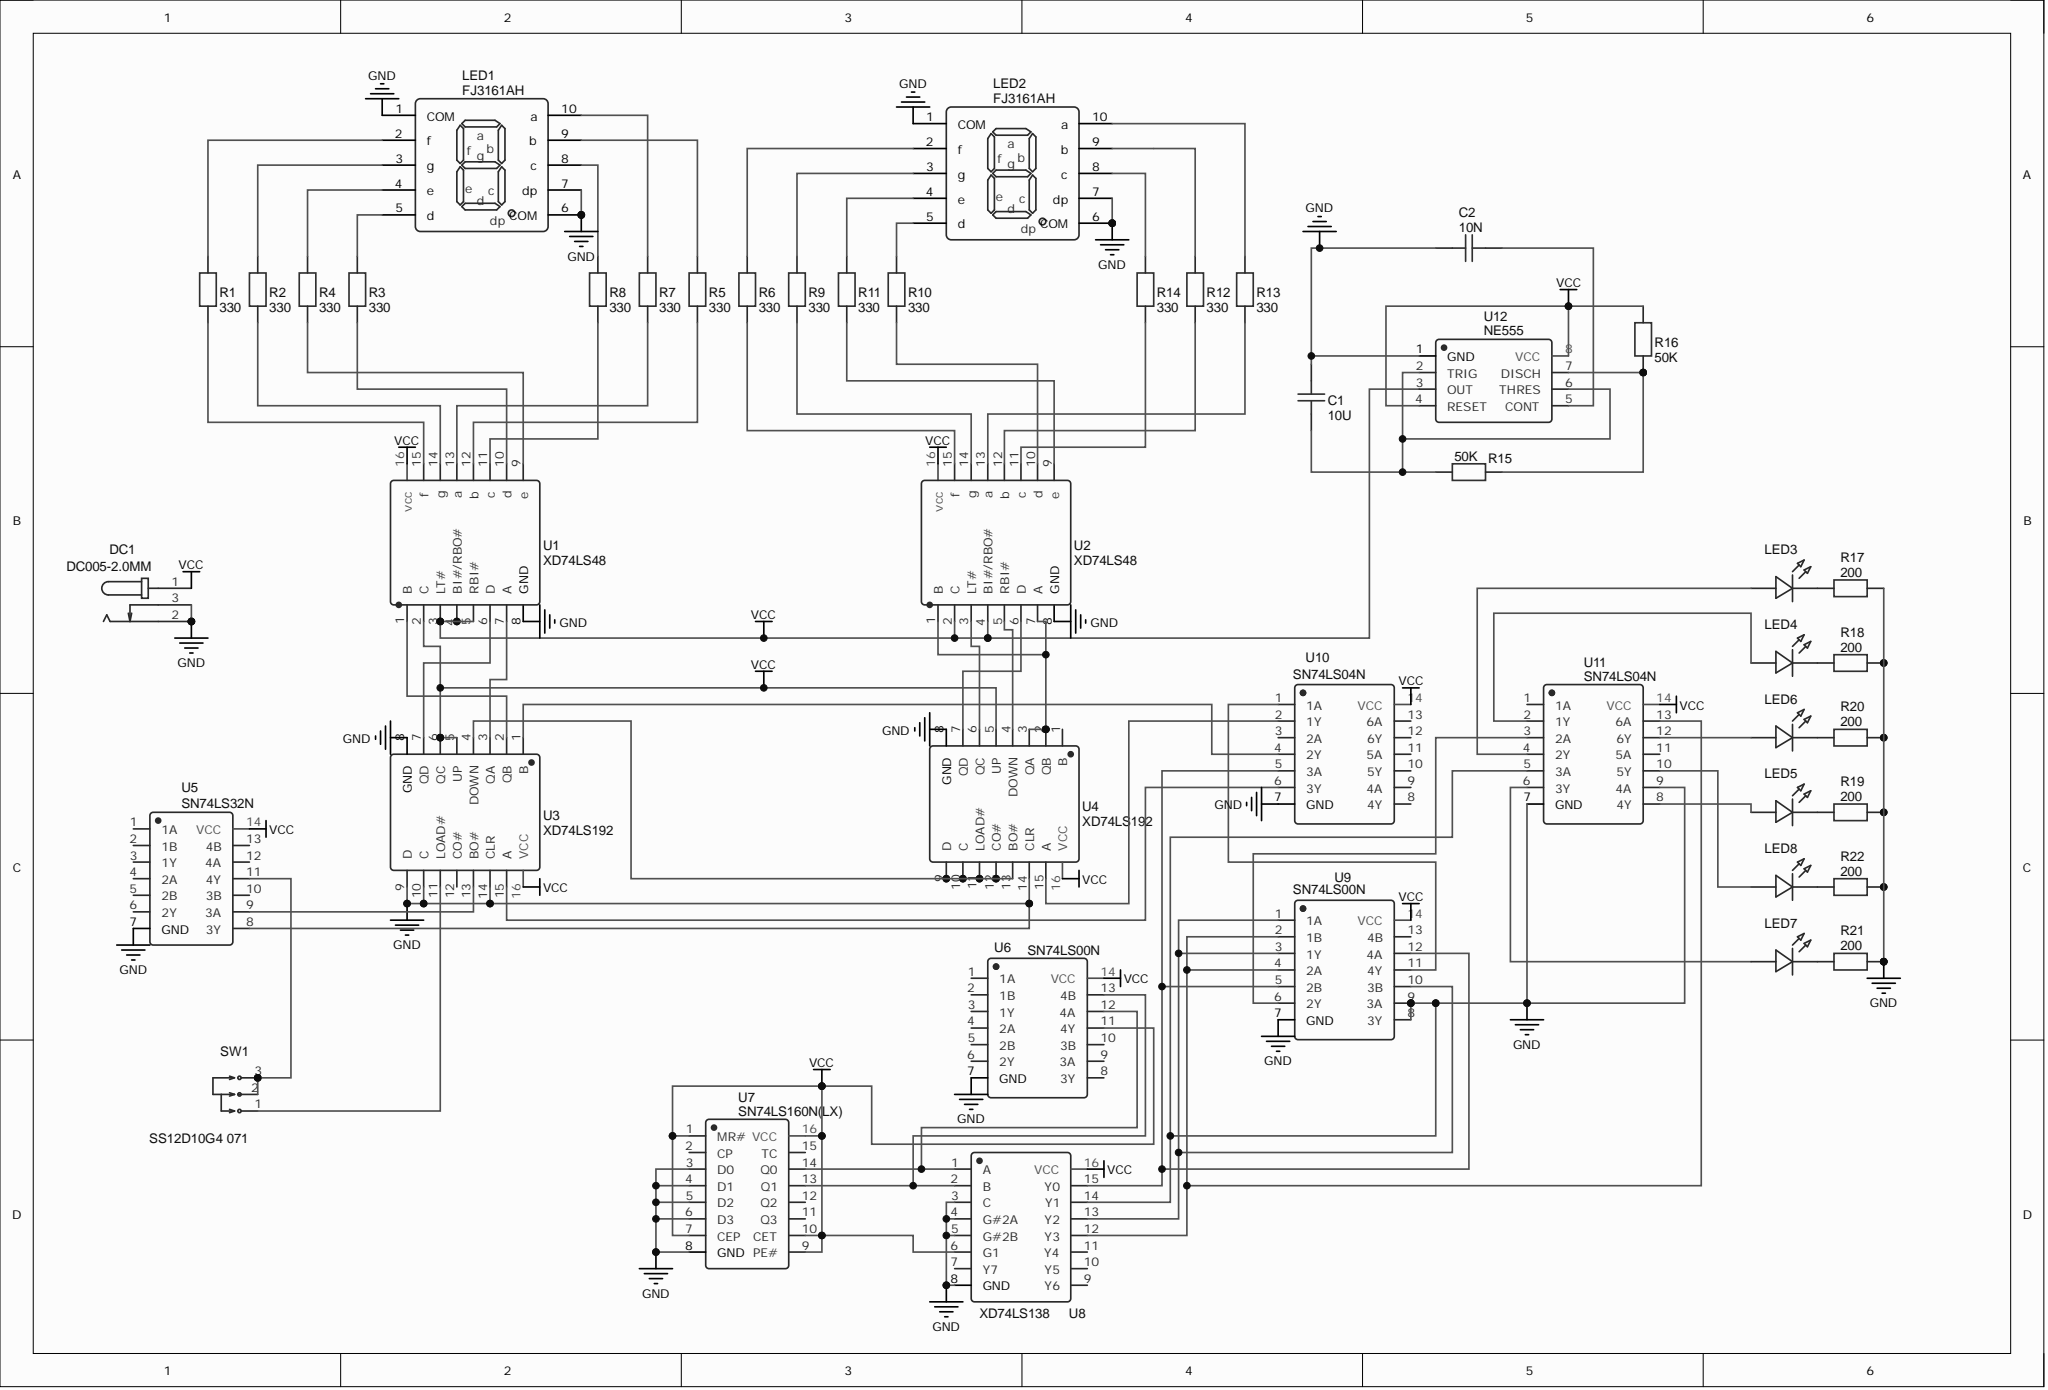Circuit board | Altium Designer | 46 parts | 66 nets
Bill of materials:
Comment,Description,Designator,Footprint,LibRef,Quantity
"10U","","C1","RAD-0.2","10U","1"
"10N","","C2","RAD-0.2","10N","1"
"DC005-2.0MM","","DC1","DC-IN-TH_DC005","DC005-2.0MM","1"
"FJ3161AH","","LED1, LED2","LED-SEG-TH_10P-L14.0-W7.5-P2.54-S5.08-TL","FJ3161AH","2"
"LED-TH-5mm_R","","LED3, LED4, LED5, LED6, LED7, LED8","LED-TH_BD5.0_RED","LED-TH-5mm_R","6"
"330","","R1, R2, R3, R4, R5, R6, R7, R8, R9, R10, R11, R12, R13, R14","R_AXIAL-0.4","330","14"
"50K","","R15, R16","R_AXIAL-0.4","50K","2"
"200","","R17, R18, R19, R20, R21, R22","R_AXIAL-0.4","200","6"
"SS12D10G4 071","","SW1","SW-TH_SHOU-HAN_SS12D10G4","SS12D10G4 071","1"
"XD74LS48","","U1, U2","DIP-16_L19.3-W6.4-P2.54-LS7.6-BL","XD74LS48","2"
"XD74LS192","","U3, U4","DIP-16_L19.3-W6.4-P2.54-LS7.6-BL","XD74LS192","2"
"SN74LS32N","","U5","PDIP-14_L19.6-W6.5-P2.54-LS7.9-BL","SN74LS32N","1"
"SN74LS00N","","U6, U9","PDIP-14_L19.7-W6.6-P2.54-LS8.3-BL","SN74LS00N","2"
"SN74LS160N(LX)","","U7","DIP-16_L22.4-W6.4-P2.54-LS8.64-BL","SN74LS160N(LX)","1"
"XD74LS138","","U8","DIP-16_L19.8-W6.5-P2.54-LS7.6-BL","XD74LS138","1"
"SN74LS04N","","U10, U11","PDIP-14_L19.7-W6.6-P2.54-LS8.3-BL","SN74LS04N","2"
"NE555","","U12","DIP-8_L9.8-W6.6-P2.54-LS7.6-BL","NE555","1"
Netlist (Protel format):
[
C1
RAD-0.2
10U



]
[
C2
RAD-0.2
10N



]
[
DC1
DC-IN-TH_DC005
DC005-2.0MM



]
[
LED1
LED-SEG-TH_10P-L14.0-W7.5-P2.54-S5.08-TL
FJ3161AH



]
[
LED2
LED-SEG-TH_10P-L14.0-W7.5-P2.54-S5.08-TL
FJ3161AH



]
[
LED3
LED-TH_BD5.0_RED
LED-TH-5mm_R



]
[
LED4
LED-TH_BD5.0_RED
LED-TH-5mm_R



]
[
LED5
LED-TH_BD5.0_RED
LED-TH-5mm_R



]
[
LED6
LED-TH_BD5.0_RED
LED-TH-5mm_R



]
[
LED7
LED-TH_BD5.0_RED
LED-TH-5mm_R



]
[
LED8
LED-TH_BD5.0_RED
LED-TH-5mm_R



]
[
R1
R_AXIAL-0.4
330



]
[
R2
R_AXIAL-0.4
330



]
[
R3
R_AXIAL-0.4
330



]
[
R4
R_AXIAL-0.4
330



]
[
R5
R_AXIAL-0.4
330



]
[
R6
R_AXIAL-0.4
330



]
[
R7
R_AXIAL-0.4
330



]
[
R8
R_AXIAL-0.4
330



]
[
R9
R_AXIAL-0.4
330



]
[
R10
R_AXIAL-0.4
330



]
[
R11
R_AXIAL-0.4
330



]
[
R12
R_AXIAL-0.4
330



]
[
R13
R_AXIAL-0.4
330



]
[
R14
R_AXIAL-0.4
330



]
[
R15
R_AXIAL-0.4
50K



]
[
R16
R_AXIAL-0.4
50K



]
[
R17
R_AXIAL-0.4
200



]
[
R18
R_AXIAL-0.4
200



]
[
R19
R_AXIAL-0.4
200



]
[
R20
R_AXIAL-0.4
200



]
[
R21
R_AXIAL-0.4
200



]
[
R22
R_AXIAL-0.4
200



]
[
SW1
SW-TH_SHOU-HAN_SS12D10G4
SS12D10G4 071



]
[
U1
DIP-16_L19.3-W6.4-P2.54-LS7.6-BL
XD74LS48



]
[
U2
DIP-16_L19.3-W6.4-P2.54-LS7.6-BL
XD74LS48



]
[
U3
DIP-16_L19.3-W6.4-P2.54-LS7.6-BL
XD74LS192



]
[
U4
DIP-16_L19.3-W6.4-P2.54-LS7.6-BL
XD74LS192



]
[
U5
PDIP-14_L19.6-W6.5-P2.54-LS7.9-BL
SN74LS32N



]
[
U6
PDIP-14_L19.7-W6.6-P2.54-LS8.3-BL
SN74LS00N



]
[
U7
DIP-16_L22.4-W6.4-P2.54-LS8.64-BL
SN74LS160N(LX)



]
[
U8
DIP-16_L19.8-W6.5-P2.54-LS7.6-BL
XD74LS138



]
[
U9
PDIP-14_L19.7-W6.6-P2.54-LS8.3-BL
SN74LS00N



]
[
U10
PDIP-14_L19.7-W6.6-P2.54-LS8.3-BL
SN74LS04N



]
[
U11
PDIP-14_L19.7-W6.6-P2.54-LS8.3-BL
SN74LS04N



]
[
U12
DIP-8_L9.8-W6.6-P2.54-LS7.6-BL
NE555



]
(
VCC
DC1-1
R16-1
U1-2
U1-3
U1-4
U1-5
U1-16
U2-2
U2-4
U2-16
U3-5
U3-6
U3-16
U4-5
U4-16
U5-14
U6-11
U6-14
U7-1
U7-7
U7-9
U7-10
U7-16
U8-6
U8-16
U9-14
U10-14
U11-14
U12-3
U12-4
U12-8
)
(
NetU9_11
U9-11
U10-1
)
(
NetU9_6
U9-6
U11-3
)
(
NetU8_15
U8-15
U9-5
U9-12
U10-5
)
(
NetU8_13
U8-13
U9-1
U9-3
U9-10
)
(
NetU8_12
U8-12
U9-2
U9-4
U11-13
)
(
NetU6_13
U6-13
U7-13
U8-2
)
(
NetU6_12
U6-12
U7-14
U8-1
)
(
NetU4_15
U4-15
U10-2
)
(
NetU3_15
U3-15
U10-6
)
(
NetU3_13
U3-13
U5-9
)
(
NetU3_4
U3-4
U4-9
U4-10
U4-11
U4-12
U4-13
)
(
NetU3_1
U3-1
U10-4
)
(
NetU2_6
U2-6
U4-7
)
(
NetU2_5
U2-5
U4-4
)
(
NetU2_3
U2-3
U4-6
)
(
NetU2_1
U2-1
U2-7
U4-2
U4-3
)
(
NetU1_7
U1-7
U3-3
)
(
NetU1_6
U1-6
U3-7
)
(
NetU1_1
U1-1
U3-2
)
(
NetSW1_2
SW1-2
SW1-3
U5-11
)
(
NetSW1_1
SW1-1
U3-11
)
(
NetR15_1
R15-1
R16-2
U12-7
)
(
NetR14_1
R14-1
U2-11
)
(
NetR13_1
R13-1
U2-13
)
(
NetR12_1
R12-1
U2-12
)
(
NetR11_1
R11-1
U2-9
)
(
NetR10_1
R10-1
U2-10
)
(
NetR9_1
R9-1
U2-14
)
(
NetR8_1
R8-1
U1-11
)
(
NetR7_1
R7-1
U1-13
)
(
NetR6_1
R6-1
U2-15
)
(
NetR5_1
R5-1
U1-12
)
(
NetR4_1
R4-1
U1-9
)
(
NetR3_1
R3-1
U1-10
)
(
NetR2_1
R2-1
U1-14
)
(
NetR1_1
R1-1
U1-15
)
(
NetLED8_2
LED8-2
R22-1
)
(
NetLED8_1
LED8-1
U11-10
)
(
NetLED7_2
LED7-2
R21-1
)
(
NetLED7_1
LED7-1
U11-6
)
(
NetLED6_2
LED6-2
R20-1
)
(
NetLED6_1
LED6-1
U11-12
)
(
NetLED5_2
LED5-2
R19-1
)
(
NetLED5_1
LED5-1
U11-8
)
(
NetLED4_2
LED4-2
R18-1
)
(
NetLED4_1
LED4-1
U11-2
)
(
NetLED3_2
LED3-2
R17-1
)
(
NetLED3_1
LED3-1
U11-4
)
(
NetLED2_10
LED2-10
R13-2
)
(
NetLED2_9
LED2-9
R12-2
)
(
NetLED2_8
LED2-8
R14-2
)
(
NetLED2_5
LED2-5
R10-2
)
(
NetLED2_4
LED2-4
R11-2
)
(
NetLED2_3
LED2-3
R9-2
)
(
NetLED2_2
LED2-2
R6-2
)
(
NetLED1_10
LED1-10
R7-2
)
(
NetLED1_9
LED1-9
R5-2
)
(
NetLED1_8
LED1-8
R8-2
)
(
NetLED1_5
LED1-5
R3-2
)
(
NetLED1_4
LED1-4
R4-2
)
(
NetLED1_3
LED1-3
R2-2
)
(
NetLED1_2
LED1-2
R1-2
)
(
NetC2_1
C2-1
U12-5
)
(
NetC1_1
C1-1
R15-2
U12-2
U12-6
)
(
GND
C1-2
C2-2
DC1-2
DC1-3
LED1-1
LED1-6
LED1-7
LED2-1
LED2-6
LED2-7
R17-2
R18-2
R19-2
R20-2
R21-2
R22-2
U1-8
U2-8
U3-8
U3-9
U3-10
U3-14
U4-8
U4-14
U5-7
U5-8
U6-7
U7-3
U7-4
U7-5
U7-6
U7-8
U8-3
U8-4
U8-5
U8-8
U8-14
U9-7
U9-8
U9-9
U10-7
U11-5
U11-7
U11-9
U12-1
)